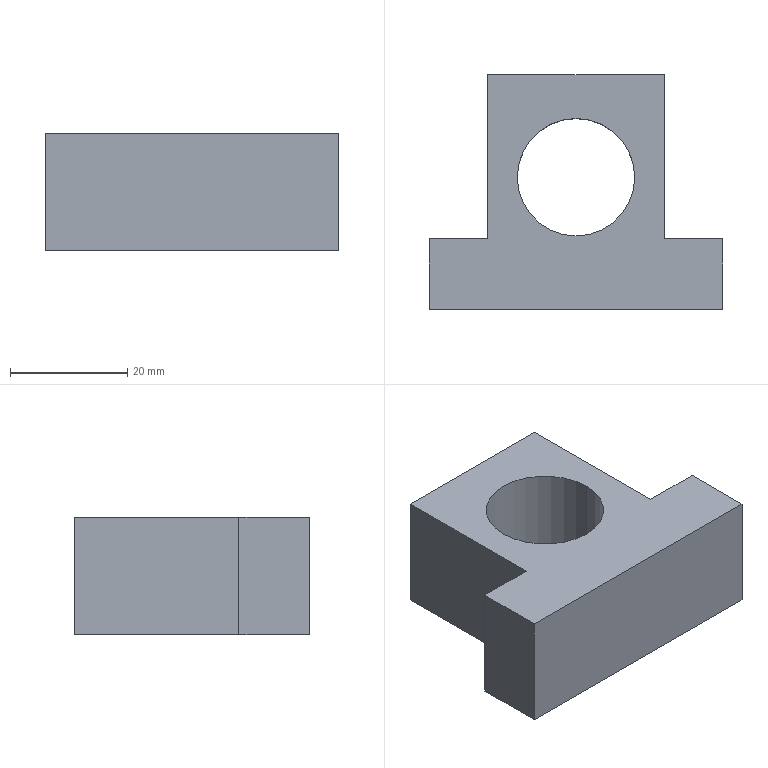Part | SolidWorks | features ICE 2, Extrusion 1 | 1 solid | 12 faces | box 50 x 40 x 20 mm | volume 22517 mm3 | plane 10 | cylinder 2 | commonest cylinder face diameters 20 x2
STEP:
#1=CARTESIAN_POINT('',(-10.,2.5,0.));
#2=VERTEX_POINT('',#1);
#3=CARTESIAN_POINT('',(10.,2.5,0.));
#4=VERTEX_POINT('',#3);
#5=CARTESIAN_POINT('',(0.,2.5,0.));
#6=DIRECTION('',(0.,0.,1.));
#7=DIRECTION('',(1.,0.,0.));
#8=AXIS2_PLACEMENT_3D('',#5,#6,#7);
#9=CIRCLE('',#8,10.);
#10=EDGE_CURVE('',#2,#4,#9,.T.);
#11=ORIENTED_EDGE('',*,*,#10,.F.);
#12=CARTESIAN_POINT('',(-10.,2.5,20.));
#13=VERTEX_POINT('',#12);
#14=CARTESIAN_POINT('',(-10.,2.5,0.));
#15=DIRECTION('',(0.,0.,1.));
#16=VECTOR('',#15,1000.);
#17=LINE('',#14,#16);
#18=EDGE_CURVE('',#2,#13,#17,.T.);
#19=ORIENTED_EDGE('',*,*,#18,.T.);
#20=CARTESIAN_POINT('',(10.,2.5,20.));
#21=VERTEX_POINT('',#20);
#22=CARTESIAN_POINT('',(0.,2.5,20.));
#23=DIRECTION('',(0.,0.,1.));
#24=DIRECTION('',(1.,0.,0.));
#25=AXIS2_PLACEMENT_3D('',#22,#23,#24);
#26=CIRCLE('',#25,10.);
#27=EDGE_CURVE('',#13,#21,#26,.T.);
#28=ORIENTED_EDGE('',*,*,#27,.T.);
#29=CARTESIAN_POINT('',(10.,2.5,0.));
#30=DIRECTION('',(0.,0.,1.));
#31=VECTOR('',#30,1000.);
#32=LINE('',#29,#31);
#33=EDGE_CURVE('',#4,#21,#32,.T.);
#34=ORIENTED_EDGE('',*,*,#33,.F.);
#35=EDGE_LOOP('',(#11,#19,#28,#34));
#36=FACE_OUTER_BOUND('',#35,.T.);
#37=CARTESIAN_POINT('',(0.,2.5,0.));
#38=DIRECTION('',(0.,0.,1.));
#39=DIRECTION('',(1.,0.,0.));
#40=AXIS2_PLACEMENT_3D('',#37,#38,#39);
#41=CYLINDRICAL_SURFACE('',#40,10.);
#42=ADVANCED_FACE('',(#36),#41,.F.);
#43=CARTESIAN_POINT('',(25.,-20.,0.));
#44=VERTEX_POINT('',#43);
#45=CARTESIAN_POINT('',(25.,-8.,0.));
#46=VERTEX_POINT('',#45);
#47=CARTESIAN_POINT('',(25.,-20.,0.));
#48=DIRECTION('',(0.,1.,0.));
#49=VECTOR('',#48,1000.);
#50=LINE('',#47,#49);
#51=EDGE_CURVE('',#44,#46,#50,.T.);
#52=ORIENTED_EDGE('',*,*,#51,.T.);
#53=CARTESIAN_POINT('',(25.,-8.,20.));
#54=VERTEX_POINT('',#53);
#55=CARTESIAN_POINT('',(25.,-8.,0.));
#56=DIRECTION('',(0.,0.,1.));
#57=VECTOR('',#56,1000.);
#58=LINE('',#55,#57);
#59=EDGE_CURVE('',#46,#54,#58,.T.);
#60=ORIENTED_EDGE('',*,*,#59,.T.);
#61=CARTESIAN_POINT('',(25.,-20.,20.));
#62=VERTEX_POINT('',#61);
#63=CARTESIAN_POINT('',(25.,-20.,20.));
#64=DIRECTION('',(0.,1.,0.));
#65=VECTOR('',#64,1000.);
#66=LINE('',#63,#65);
#67=EDGE_CURVE('',#62,#54,#66,.T.);
#68=ORIENTED_EDGE('',*,*,#67,.F.);
#69=CARTESIAN_POINT('',(25.,-20.,20.));
#70=DIRECTION('',(0.,0.,-1.));
#71=VECTOR('',#70,1000.);
#72=LINE('',#69,#71);
#73=EDGE_CURVE('',#62,#44,#72,.T.);
#74=ORIENTED_EDGE('',*,*,#73,.T.);
#75=EDGE_LOOP('',(#52,#60,#68,#74));
#76=FACE_OUTER_BOUND('',#75,.T.);
#77=CARTESIAN_POINT('',(25.,-20.,20.));
#78=DIRECTION('',(-1.,0.,0.));
#79=DIRECTION('',(0.,0.,1.));
#80=AXIS2_PLACEMENT_3D('',#77,#78,#79);
#81=PLANE('',#80);
#82=ADVANCED_FACE('',(#76),#81,.F.);
#83=CARTESIAN_POINT('',(15.,20.,0.));
#84=VERTEX_POINT('',#83);
#85=CARTESIAN_POINT('',(-15.,20.,0.));
#86=VERTEX_POINT('',#85);
#87=CARTESIAN_POINT('',(-25.,20.,0.));
#88=DIRECTION('',(-1.,0.,0.));
#89=VECTOR('',#88,1000.);
#90=LINE('',#87,#89);
#91=EDGE_CURVE('',#84,#86,#90,.T.);
#92=ORIENTED_EDGE('',*,*,#91,.T.);
#93=CARTESIAN_POINT('',(-15.,20.,20.));
#94=VERTEX_POINT('',#93);
#95=CARTESIAN_POINT('',(-15.,20.,0.));
#96=DIRECTION('',(0.,0.,1.));
#97=VECTOR('',#96,1000.);
#98=LINE('',#95,#97);
#99=EDGE_CURVE('',#86,#94,#98,.T.);
#100=ORIENTED_EDGE('',*,*,#99,.T.);
#101=CARTESIAN_POINT('',(15.,20.,20.));
#102=VERTEX_POINT('',#101);
#103=CARTESIAN_POINT('',(-25.,20.,20.));
#104=DIRECTION('',(-1.,0.,0.));
#105=VECTOR('',#104,1000.);
#106=LINE('',#103,#105);
#107=EDGE_CURVE('',#102,#94,#106,.T.);
#108=ORIENTED_EDGE('',*,*,#107,.F.);
#109=CARTESIAN_POINT('',(15.,20.,0.));
#110=DIRECTION('',(0.,0.,1.));
#111=VECTOR('',#110,1000.);
#112=LINE('',#109,#111);
#113=EDGE_CURVE('',#84,#102,#112,.T.);
#114=ORIENTED_EDGE('',*,*,#113,.F.);
#115=EDGE_LOOP('',(#92,#100,#108,#114));
#116=FACE_OUTER_BOUND('',#115,.T.);
#117=CARTESIAN_POINT('',(-25.,20.,20.));
#118=DIRECTION('',(0.,-1.,0.));
#119=DIRECTION('',(0.,0.,-1.));
#120=AXIS2_PLACEMENT_3D('',#117,#118,#119);
#121=PLANE('',#120);
#122=ADVANCED_FACE('',(#116),#121,.F.);
#123=CARTESIAN_POINT('',(-25.,-8.,20.));
#124=VERTEX_POINT('',#123);
#125=CARTESIAN_POINT('',(-25.,-20.,20.));
#126=VERTEX_POINT('',#125);
#127=CARTESIAN_POINT('',(-25.,-20.,20.));
#128=DIRECTION('',(0.,-1.,0.));
#129=VECTOR('',#128,1000.);
#130=LINE('',#127,#129);
#131=EDGE_CURVE('',#124,#126,#130,.T.);
#132=ORIENTED_EDGE('',*,*,#131,.F.);
#133=CARTESIAN_POINT('',(-25.,-8.,0.));
#134=VERTEX_POINT('',#133);
#135=CARTESIAN_POINT('',(-25.,-8.,0.));
#136=DIRECTION('',(0.,0.,1.));
#137=VECTOR('',#136,1000.);
#138=LINE('',#135,#137);
#139=EDGE_CURVE('',#134,#124,#138,.T.);
#140=ORIENTED_EDGE('',*,*,#139,.F.);
#141=CARTESIAN_POINT('',(-25.,-20.,0.));
#142=VERTEX_POINT('',#141);
#143=CARTESIAN_POINT('',(-25.,-20.,0.));
#144=DIRECTION('',(0.,-1.,0.));
#145=VECTOR('',#144,1000.);
#146=LINE('',#143,#145);
#147=EDGE_CURVE('',#134,#142,#146,.T.);
#148=ORIENTED_EDGE('',*,*,#147,.T.);
#149=CARTESIAN_POINT('',(-25.,-20.,20.));
#150=DIRECTION('',(0.,0.,-1.));
#151=VECTOR('',#150,1000.);
#152=LINE('',#149,#151);
#153=EDGE_CURVE('',#126,#142,#152,.T.);
#154=ORIENTED_EDGE('',*,*,#153,.F.);
#155=EDGE_LOOP('',(#132,#140,#148,#154));
#156=FACE_OUTER_BOUND('',#155,.T.);
#157=CARTESIAN_POINT('',(-25.,-20.,20.));
#158=DIRECTION('',(1.,0.,0.));
#159=DIRECTION('',(0.,0.,-1.));
#160=AXIS2_PLACEMENT_3D('',#157,#158,#159);
#161=PLANE('',#160);
#162=ADVANCED_FACE('',(#156),#161,.F.);
#163=CARTESIAN_POINT('',(-25.,-20.,0.));
#164=DIRECTION('',(1.,0.,0.));
#165=VECTOR('',#164,1000.);
#166=LINE('',#163,#165);
#167=EDGE_CURVE('',#142,#44,#166,.T.);
#168=ORIENTED_EDGE('',*,*,#167,.T.);
#169=ORIENTED_EDGE('',*,*,#73,.F.);
#170=CARTESIAN_POINT('',(-25.,-20.,20.));
#171=DIRECTION('',(1.,0.,0.));
#172=VECTOR('',#171,1000.);
#173=LINE('',#170,#172);
#174=EDGE_CURVE('',#126,#62,#173,.T.);
#175=ORIENTED_EDGE('',*,*,#174,.F.);
#176=ORIENTED_EDGE('',*,*,#153,.T.);
#177=EDGE_LOOP('',(#168,#169,#175,#176));
#178=FACE_OUTER_BOUND('',#177,.T.);
#179=CARTESIAN_POINT('',(-25.,-20.,20.));
#180=DIRECTION('',(0.,1.,0.));
#181=DIRECTION('',(0.,0.,1.));
#182=AXIS2_PLACEMENT_3D('',#179,#180,#181);
#183=PLANE('',#182);
#184=ADVANCED_FACE('',(#178),#183,.F.);
#185=CARTESIAN_POINT('',(0.,2.5,20.));
#186=DIRECTION('',(0.,0.,1.));
#187=DIRECTION('',(1.,0.,0.));
#188=AXIS2_PLACEMENT_3D('',#185,#186,#187);
#189=CIRCLE('',#188,10.);
#190=EDGE_CURVE('',#21,#13,#189,.T.);
#191=ORIENTED_EDGE('',*,*,#190,.F.);
#192=ORIENTED_EDGE('',*,*,#27,.F.);
#193=EDGE_LOOP('',(#191,#192));
#194=FACE_BOUND('',#193,.T.);
#195=ORIENTED_EDGE('',*,*,#107,.T.);
#196=CARTESIAN_POINT('',(-15.,-8.,20.));
#197=VERTEX_POINT('',#196);
#198=CARTESIAN_POINT('',(-15.,20.,20.));
#199=DIRECTION('',(0.,1.,0.));
#200=VECTOR('',#199,1000.);
#201=LINE('',#198,#200);
#202=EDGE_CURVE('',#197,#94,#201,.T.);
#203=ORIENTED_EDGE('',*,*,#202,.F.);
#204=CARTESIAN_POINT('',(-25.,-8.,20.));
#205=DIRECTION('',(1.,0.,0.));
#206=VECTOR('',#205,1000.);
#207=LINE('',#204,#206);
#208=EDGE_CURVE('',#124,#197,#207,.T.);
#209=ORIENTED_EDGE('',*,*,#208,.F.);
#210=ORIENTED_EDGE('',*,*,#131,.T.);
#211=ORIENTED_EDGE('',*,*,#174,.T.);
#212=ORIENTED_EDGE('',*,*,#67,.T.);
#213=CARTESIAN_POINT('',(15.,-8.,20.));
#214=VERTEX_POINT('',#213);
#215=CARTESIAN_POINT('',(25.,-8.,20.));
#216=DIRECTION('',(1.,0.,0.));
#217=VECTOR('',#216,1000.);
#218=LINE('',#215,#217);
#219=EDGE_CURVE('',#214,#54,#218,.T.);
#220=ORIENTED_EDGE('',*,*,#219,.F.);
#221=CARTESIAN_POINT('',(15.,20.,20.));
#222=DIRECTION('',(0.,-1.,0.));
#223=VECTOR('',#222,1000.);
#224=LINE('',#221,#223);
#225=EDGE_CURVE('',#102,#214,#224,.T.);
#226=ORIENTED_EDGE('',*,*,#225,.F.);
#227=EDGE_LOOP('',(#195,#203,#209,#210,#211,#212,#220,#226));
#228=FACE_OUTER_BOUND('',#227,.T.);
#229=CARTESIAN_POINT('',(0.,0.,20.));
#230=DIRECTION('',(0.,0.,-1.));
#231=DIRECTION('',(-1.,0.,0.));
#232=AXIS2_PLACEMENT_3D('',#229,#230,#231);
#233=PLANE('',#232);
#234=ADVANCED_FACE('',(#194,#228),#233,.F.);
#235=CARTESIAN_POINT('',(-15.,-8.,0.));
#236=VERTEX_POINT('',#235);
#237=CARTESIAN_POINT('',(-15.,20.,0.));
#238=DIRECTION('',(0.,1.,0.));
#239=VECTOR('',#238,1000.);
#240=LINE('',#237,#239);
#241=EDGE_CURVE('',#236,#86,#240,.T.);
#242=ORIENTED_EDGE('',*,*,#241,.T.);
#243=ORIENTED_EDGE('',*,*,#91,.F.);
#244=CARTESIAN_POINT('',(15.,-8.,0.));
#245=VERTEX_POINT('',#244);
#246=CARTESIAN_POINT('',(15.,20.,0.));
#247=DIRECTION('',(0.,-1.,0.));
#248=VECTOR('',#247,1000.);
#249=LINE('',#246,#248);
#250=EDGE_CURVE('',#84,#245,#249,.T.);
#251=ORIENTED_EDGE('',*,*,#250,.T.);
#252=CARTESIAN_POINT('',(25.,-8.,0.));
#253=DIRECTION('',(1.,0.,0.));
#254=VECTOR('',#253,1000.);
#255=LINE('',#252,#254);
#256=EDGE_CURVE('',#245,#46,#255,.T.);
#257=ORIENTED_EDGE('',*,*,#256,.T.);
#258=ORIENTED_EDGE('',*,*,#51,.F.);
#259=ORIENTED_EDGE('',*,*,#167,.F.);
#260=ORIENTED_EDGE('',*,*,#147,.F.);
#261=CARTESIAN_POINT('',(-25.,-8.,0.));
#262=DIRECTION('',(1.,0.,0.));
#263=VECTOR('',#262,1000.);
#264=LINE('',#261,#263);
#265=EDGE_CURVE('',#134,#236,#264,.T.);
#266=ORIENTED_EDGE('',*,*,#265,.T.);
#267=EDGE_LOOP('',(#242,#243,#251,#257,#258,#259,#260,#266));
#268=FACE_OUTER_BOUND('',#267,.T.);
#269=CARTESIAN_POINT('',(0.,2.5,0.));
#270=DIRECTION('',(0.,0.,1.));
#271=DIRECTION('',(1.,0.,0.));
#272=AXIS2_PLACEMENT_3D('',#269,#270,#271);
#273=CIRCLE('',#272,10.);
#274=EDGE_CURVE('',#4,#2,#273,.T.);
#275=ORIENTED_EDGE('',*,*,#274,.T.);
#276=ORIENTED_EDGE('',*,*,#10,.T.);
#277=EDGE_LOOP('',(#275,#276));
#278=FACE_BOUND('',#277,.T.);
#279=CARTESIAN_POINT('',(0.,0.,0.));
#280=DIRECTION('',(0.,0.,-1.));
#281=DIRECTION('',(-1.,0.,0.));
#282=AXIS2_PLACEMENT_3D('',#279,#280,#281);
#283=PLANE('',#282);
#284=ADVANCED_FACE('',(#268,#278),#283,.T.);
#285=ORIENTED_EDGE('',*,*,#18,.F.);
#286=ORIENTED_EDGE('',*,*,#274,.F.);
#287=ORIENTED_EDGE('',*,*,#33,.T.);
#288=ORIENTED_EDGE('',*,*,#190,.T.);
#289=EDGE_LOOP('',(#285,#286,#287,#288));
#290=FACE_OUTER_BOUND('',#289,.T.);
#291=CARTESIAN_POINT('',(0.,2.5,0.));
#292=DIRECTION('',(0.,0.,1.));
#293=DIRECTION('',(1.,0.,0.));
#294=AXIS2_PLACEMENT_3D('',#291,#292,#293);
#295=CYLINDRICAL_SURFACE('',#294,10.);
#296=ADVANCED_FACE('',(#290),#295,.F.);
#297=ORIENTED_EDGE('',*,*,#219,.T.);
#298=ORIENTED_EDGE('',*,*,#59,.F.);
#299=ORIENTED_EDGE('',*,*,#256,.F.);
#300=CARTESIAN_POINT('',(15.,-8.,0.));
#301=DIRECTION('',(0.,0.,1.));
#302=VECTOR('',#301,1000.);
#303=LINE('',#300,#302);
#304=EDGE_CURVE('',#245,#214,#303,.T.);
#305=ORIENTED_EDGE('',*,*,#304,.T.);
#306=EDGE_LOOP('',(#297,#298,#299,#305));
#307=FACE_OUTER_BOUND('',#306,.T.);
#308=CARTESIAN_POINT('',(25.,-8.,0.));
#309=DIRECTION('',(0.,-1.,0.));
#310=DIRECTION('',(0.,0.,-1.));
#311=AXIS2_PLACEMENT_3D('',#308,#309,#310);
#312=PLANE('',#311);
#313=ADVANCED_FACE('',(#307),#312,.F.);
#314=ORIENTED_EDGE('',*,*,#225,.T.);
#315=ORIENTED_EDGE('',*,*,#304,.F.);
#316=ORIENTED_EDGE('',*,*,#250,.F.);
#317=ORIENTED_EDGE('',*,*,#113,.T.);
#318=EDGE_LOOP('',(#314,#315,#316,#317));
#319=FACE_OUTER_BOUND('',#318,.T.);
#320=CARTESIAN_POINT('',(15.,20.,0.));
#321=DIRECTION('',(-1.,0.,0.));
#322=DIRECTION('',(0.,-1.,0.));
#323=AXIS2_PLACEMENT_3D('',#320,#321,#322);
#324=PLANE('',#323);
#325=ADVANCED_FACE('',(#319),#324,.F.);
#326=ORIENTED_EDGE('',*,*,#202,.T.);
#327=ORIENTED_EDGE('',*,*,#99,.F.);
#328=ORIENTED_EDGE('',*,*,#241,.F.);
#329=CARTESIAN_POINT('',(-15.,-8.,0.));
#330=DIRECTION('',(0.,0.,1.));
#331=VECTOR('',#330,1000.);
#332=LINE('',#329,#331);
#333=EDGE_CURVE('',#236,#197,#332,.T.);
#334=ORIENTED_EDGE('',*,*,#333,.T.);
#335=EDGE_LOOP('',(#326,#327,#328,#334));
#336=FACE_OUTER_BOUND('',#335,.T.);
#337=CARTESIAN_POINT('',(-15.,20.,0.));
#338=DIRECTION('',(1.,0.,0.));
#339=DIRECTION('',(0.,1.,0.));
#340=AXIS2_PLACEMENT_3D('',#337,#338,#339);
#341=PLANE('',#340);
#342=ADVANCED_FACE('',(#336),#341,.F.);
#343=ORIENTED_EDGE('',*,*,#208,.T.);
#344=ORIENTED_EDGE('',*,*,#333,.F.);
#345=ORIENTED_EDGE('',*,*,#265,.F.);
#346=ORIENTED_EDGE('',*,*,#139,.T.);
#347=EDGE_LOOP('',(#343,#344,#345,#346));
#348=FACE_OUTER_BOUND('',#347,.T.);
#349=CARTESIAN_POINT('',(-25.,-8.,0.));
#350=DIRECTION('',(0.,-1.,0.));
#351=DIRECTION('',(0.,0.,-1.));
#352=AXIS2_PLACEMENT_3D('',#349,#350,#351);
#353=PLANE('',#352);
#354=ADVANCED_FACE('',(#348),#353,.F.);
#355=CLOSED_SHELL('',(#42,#82,#122,#162,#184,#234,#284,#296,#313,#325,#342,#354));
#356=MANIFOLD_SOLID_BREP('',#355);
#357=CARTESIAN_POINT('',(0.,0.,0.));
#358=DIRECTION('',(0.,0.,1.));
#359=DIRECTION('',(1.,0.,0.));
#360=AXIS2_PLACEMENT_3D('',#357,#358,#359);
#361=(LENGTH_UNIT()NAMED_UNIT(*)SI_UNIT(.MILLI.,.METRE.));
#362=UNCERTAINTY_MEASURE_WITH_UNIT(LENGTH_MEASURE(0.00001),#361,'','');
#363=(NAMED_UNIT(*)PLANE_ANGLE_UNIT()SI_UNIT($,.RADIAN.));
#364=(NAMED_UNIT(*)SI_UNIT($,.STERADIAN.)SOLID_ANGLE_UNIT());
#365=(GEOMETRIC_REPRESENTATION_CONTEXT(3)GLOBAL_UNCERTAINTY_ASSIGNED_CONTEXT((#362))GLOBAL_UNIT_ASSIGNED_CONTEXT((#361,#363,#364))REPRESENTATION_CONTEXT('',''));
#366=ADVANCED_BREP_SHAPE_REPRESENTATION('',(#356,#360),#365);